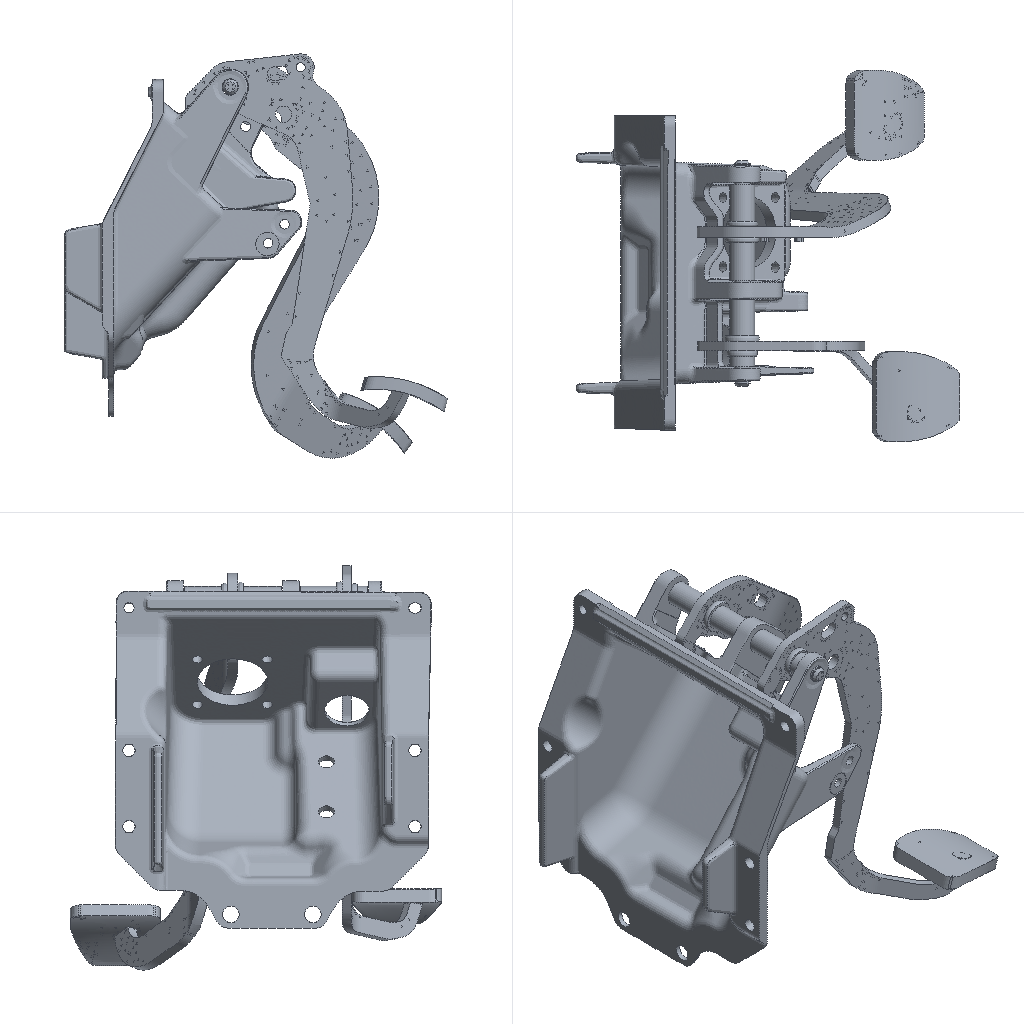Simulation study | nastran
Set-up summary:
category,name,step,type,value,unit,region
solver,nx_nastran
units,not stated in the deck,,not stated
analysis,deck,,modal,modal
analysis,solution,,SOL,103
load_step,SUBCASE 1,1,SUBCASE,SPC=1 LOAD=None
mesh,nodes,,,225553
mesh,elements,,,488318
element_type,CHEXA,,unverified,78992
element_type,CPENTA,,unverified,2405
element_type,CTETRA,,solid,488318
load,load commands in deck,,count,0
bc,support commands in deck,,count,8
check,setup vs results,,match,"every grid point's frame and coordinates and every element id; grid points of CHEXA, CPENTA, CTETRA elements"
Nastran input file, long lists of numbers shortened:
$$------------------------------------------------------------------------------$
$$                                                                              $
$$ NASTRAN Input Deck Generated by HyperMesh Version  :10.0buil                 $
$$ Generated using HyperMesh-Nastran Template Version : 10.0build60
$$                                                                              $
$$   Template:  general                                                         $
$$                                                                              $
$$------------------------------------------------------------------------------$
$$------------------------------------------------------------------------------$
$$                      Executive Control Cards                                 $
$$------------------------------------------------------------------------------$
SOL 103
CEND
$$------------------------------------------------------------------------------$
$$                      Case Control Cards                                      $
$$------------------------------------------------------------------------------$
  DISPLACEMENT = ALL
  ESE = ALL
$
$HMNAME LOADSTEP               1"modal"
SUBCASE       1
  LABEL=  modal
  SPC =        1
  METHOD(STRUCTURE) =        2
$$------------------------------------------------------------------------------$
$$                      Bulk Data Cards                                         $
$$------------------------------------------------------------------------------$
BEGIN BULK
PARAM,POST,-1
$$
$$  GRID Data
$$
GRID          13        -1019.28-605.268632.4837
GRID          14        -1019.28-603.268632.4837
$ (225551 more lines like these left out)
$$
$$  SPOINT Data
$$
$$
$$------------------------------------------------------------------------------$
$$             Group Definitions                                                $
$$------------------------------------------------------------------------------$
$$
$$ RBE2 Elements - Multiple dependent nodes
$$
RBE2     1606838  343215  123456  199871  199872  199873  199874  199875+
+         199876  199877  199878  199879  199880  199881  199882  199883+
+         199884  199885  199886  200499  200500  200501  200502  200503+
+         200504  200505  200506  200507  200508  200509  200510  200511+
+         200512  200513  200514  243897  243898  243899  243900  243901+
+         243902  243903  243904  243905  243906  243907  243908  243909+
+         243910  243911  243912  243913  243914  243915  243916  243917+
+         243918  243919  243920  243921  243922  243923  243924  243925+
+         243926  243927  243928  243929  243930  243931  243932  243933+
+         243934  243935  243936  243937  243938  243939  243940  243941+
+         243942  243943  243944  243945  243946  243947  243948  243949+
+         243950  243951  243952  243953  243954  243955  243956  243957+
+         243958  243959  243960  243961  243962  243963  243964  243965+
+         243966  243967  243968  243969  243970
RBE2     1606839  343216  123456  196071  196072  196073  196074  196075+
+         196076  196077  196078  196079  196080  196081  196082  196083+
+         196084  196085  196086  196087  196088  240159  240160  240161+
+         240162  240163  240164  240165  240166  240167  240168  240169+
+         240170  240171  240172  240173  240174  240175  240176  240971+
+         240972  240973  240974  240975  240976  240977  240978  240979+
+         240980  240981  240982  240983  240984  240985  240986  240987+
+         240988  240989  240990  240991  240992  240993  240994  240995+
+         240996  240997  240998  240999  241000  241001  241002  241003+
+         241004  241005  241006  241007  241008  241009  241010  241011+
+         241012  241013  241014  241015  241016  241017  241018  241019+
+         241020  241021  241022  241023  241024  241025  241026  241027+
+         241028  241029  241030  241031  241032  241033  241034  241035+
+         241036  241037  241038  241039  241040  241041  241042  241043+
+         241044  241045  241046
$ (837 more lines like these left out)
$
$HMMOVE        6
$        1606838THRU     1606851 1606853THRU     1606855
$
$
$  CHEXA Elements: First Order
$
CHEXA      74428       1   77279   77280   77267   77268   77283   77284+
+          77271   77272
CHEXA      74429       1   77283   77284   77271   77272   77287   77288+
+          77275   77276
$ (157980 more lines like these left out)
$
$HMMOVE        2
$          74428THRU       75374   75405THRU       75524   75549THRU       76481
$          74415THRU       74427   76482THRU       76492   76497THRU       76556
$ (227 more lines like these left out)
CTETRA   1605838       1  305206  238540  238539  238219
CTETRA   1605839       1  230294  331555  228598  325759
$ (488316 more lines like these left out)
$
$  CPENTA Elements 6-noded
$
CPENTA     75381       1   78038   78039   77846   78040   78041   77822
CPENTA     75382       1   78040   78041   77822   78042   78043   77823
$ (2403 more lines like these left out)
$
$HMMOVE        4
$        1605838THRU     1606837 1604838THRU     1605837 1603838THRU     1604837
$        1602838THRU     1603837 1601838THRU     1602837 1600838THRU     1601837
$ (382 more lines like these left out)
PSOLID         1      38
$$
$$------------------------------------------------------------------------------$
$$                      Material Definition Cards                               $
$$------------------------------------------------------------------------------$
$$--------------------------------------------------------------
$$ HYPERMESH TAGS
$$--------------------------------------------------------------
$$BEGIN TAGS
$$END TAGS
$$
$$  MAT1 Data
$
$HMNAME MAT                   38"steel" "MAT1"
$HWCOLOR MAT                  38       7
MAT1          38210000.0        0.29    7.80E-09
$$
$$
$$
$$------------------------------------------------------------------------------$
$ (34 more lines like these left out)
EIGRL          20.0                   10                            MASS
$$
$$  SPC Data
$$
SPC            1  343219  1234560.0
SPC            1  343218  1234560.0
SPC            1  343217  1234560.0
SPC            1  343216  1234560.0
SPC            1  343215  1234560.0
SPC            1  343222  1234560.0
SPC            1  343221  1234560.0
SPC            1  343220  1234560.0
$
ENDDATA
Results summary:
result,analysis,,,modal
result,primary field,,,eigenvectors